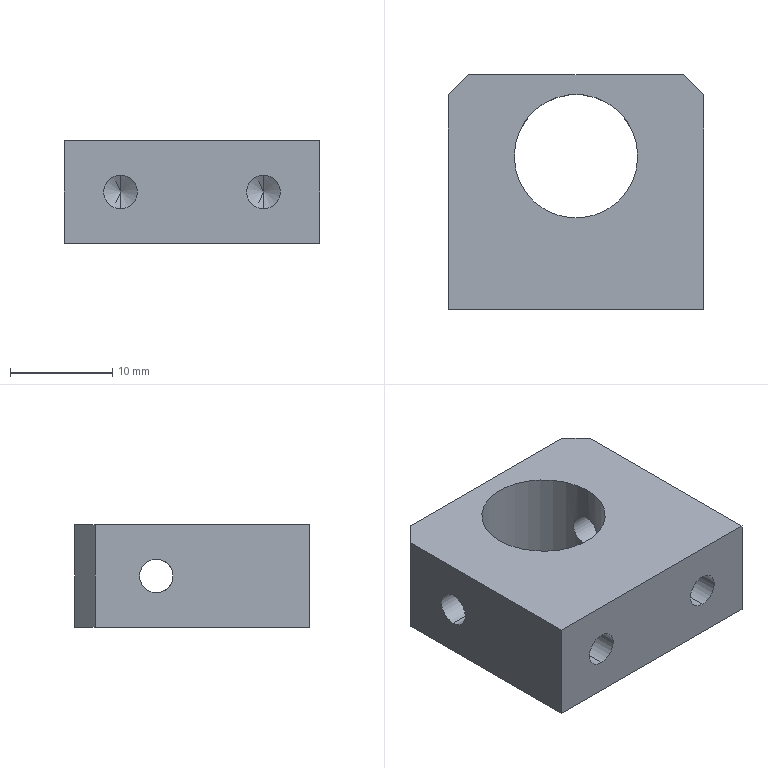Part | SolidWorks | features HoleWzd 2, Chamfer 1, Extrusion 1, ICE 1, MirrorPattern 1 | 1 solid | 22 faces | box 25 x 23 x 10 mm | volume 4270 mm3 | cylinder 10 | plane 8 | cone 4 | commonest cylinder face diameters 3.3 x8 12.1 x2
STEP:
#1=CARTESIAN_POINT('',(6.05,3.5,6.65));
#2=VERTEX_POINT('',#1);
#3=CARTESIAN_POINT('',(6.05,3.5,3.35));
#4=VERTEX_POINT('',#3);
#5=CARTESIAN_POINT('',(6.05,3.5,6.65));
#6=CARTESIAN_POINT('',(6.05,3.284,6.65));
#7=CARTESIAN_POINT('',(6.038,3.066,6.606));
#8=CARTESIAN_POINT('',(6.006,2.768,6.483));
#9=CARTESIAN_POINT('',(5.994,2.671,6.431));
#10=CARTESIAN_POINT('',(5.966,2.492,6.311));
#11=CARTESIAN_POINT('',(5.951,2.41,6.243));
#12=CARTESIAN_POINT('',(5.922,2.258,6.091));
#13=CARTESIAN_POINT('',(5.906,2.188,6.007));
#14=CARTESIAN_POINT('',(5.879,2.069,5.829));
#15=CARTESIAN_POINT('',(5.866,2.018,5.734));
#16=CARTESIAN_POINT('',(5.844,1.935,5.533));
#17=CARTESIAN_POINT('',(5.836,1.903,5.43));
#18=CARTESIAN_POINT('',(5.824,1.861,5.218));
#19=CARTESIAN_POINT('',(5.821,1.85,5.109));
#20=CARTESIAN_POINT('',(5.821,1.85,4.892));
#21=CARTESIAN_POINT('',(5.824,1.861,4.784));
#22=CARTESIAN_POINT('',(5.835,1.903,4.572));
#23=CARTESIAN_POINT('',(5.844,1.935,4.467));
#24=CARTESIAN_POINT('',(5.876,2.059,4.168));
#25=CARTESIAN_POINT('',(5.907,2.181,3.985));
#26=CARTESIAN_POINT('',(5.966,2.484,3.682));
#27=CARTESIAN_POINT('',(5.996,2.667,3.56));
#28=CARTESIAN_POINT('',(6.027,2.965,3.435));
#29=CARTESIAN_POINT('',(6.036,3.07,3.403));
#30=CARTESIAN_POINT('',(6.047,3.283,3.361));
#31=CARTESIAN_POINT('',(6.05,3.39,3.35));
#32=CARTESIAN_POINT('',(6.05,3.5,3.35));
#33=B_SPLINE_CURVE_WITH_KNOTS('',3,(#5,#6,#7,#8,#9,#10,#11,#12,#13,#14,#15,#16,#17,#18,#19,#20,#21,#22,#23,#24,#25,#26,#27,#28,#29,#30,#31,#32),.UNSPECIFIED.,.F.,.F.,(4,2,2,2,2,2,2,2,2,2,2,2,2,4),(0.005183,0.005831,0.006155,0.006479,0.006803,0.007127,0.00745,0.007774,0.008098,0.008422,0.00907,0.009717,0.01004,0.01037),.UNSPECIFIED.);
#34=EDGE_CURVE('',#2,#4,#33,.T.);
#35=ORIENTED_EDGE('',*,*,#34,.F.);
#36=CARTESIAN_POINT('',(12.5,3.5,6.65));
#37=VERTEX_POINT('',#36);
#38=CARTESIAN_POINT('',(12.5,3.5,6.65));
#39=DIRECTION('',(1.,0.,0.));
#40=VECTOR('',#39,1000.);
#41=LINE('',#38,#40);
#42=EDGE_CURVE('',#2,#37,#41,.T.);
#43=ORIENTED_EDGE('',*,*,#42,.T.);
#44=CARTESIAN_POINT('',(12.5,3.5,3.35));
#45=VERTEX_POINT('',#44);
#46=CARTESIAN_POINT('',(12.5,3.5,5.));
#47=DIRECTION('',(1.,0.,0.));
#48=DIRECTION('',(0.,0.,-1.));
#49=AXIS2_PLACEMENT_3D('',#46,#47,#48);
#50=CIRCLE('',#49,1.65);
#51=EDGE_CURVE('',#37,#45,#50,.T.);
#52=ORIENTED_EDGE('',*,*,#51,.T.);
#53=CARTESIAN_POINT('',(12.5,3.5,3.35));
#54=DIRECTION('',(1.,0.,0.));
#55=VECTOR('',#54,1000.);
#56=LINE('',#53,#55);
#57=EDGE_CURVE('',#4,#45,#56,.T.);
#58=ORIENTED_EDGE('',*,*,#57,.F.);
#59=EDGE_LOOP('',(#35,#43,#52,#58));
#60=FACE_OUTER_BOUND('',#59,.T.);
#61=CARTESIAN_POINT('',(12.5,3.5,5.));
#62=DIRECTION('',(1.,0.,0.));
#63=DIRECTION('',(0.,0.,-1.));
#64=AXIS2_PLACEMENT_3D('',#61,#62,#63);
#65=CYLINDRICAL_SURFACE('',#64,1.65);
#66=ADVANCED_FACE('',(#60),#65,.F.);
#67=CARTESIAN_POINT('',(-6.05,3.5,3.35));
#68=VERTEX_POINT('',#67);
#69=CARTESIAN_POINT('',(-6.05,3.5,6.65));
#70=VERTEX_POINT('',#69);
#71=CARTESIAN_POINT('',(-6.05,3.5,3.35));
#72=CARTESIAN_POINT('',(-6.05,3.284,3.35));
#73=CARTESIAN_POINT('',(-6.038,3.066,3.394));
#74=CARTESIAN_POINT('',(-6.006,2.768,3.517));
#75=CARTESIAN_POINT('',(-5.994,2.671,3.569));
#76=CARTESIAN_POINT('',(-5.966,2.492,3.689));
#77=CARTESIAN_POINT('',(-5.951,2.41,3.757));
#78=CARTESIAN_POINT('',(-5.922,2.258,3.909));
#79=CARTESIAN_POINT('',(-5.906,2.188,3.993));
#80=CARTESIAN_POINT('',(-5.879,2.069,4.171));
#81=CARTESIAN_POINT('',(-5.866,2.018,4.266));
#82=CARTESIAN_POINT('',(-5.844,1.935,4.467));
#83=CARTESIAN_POINT('',(-5.836,1.903,4.57));
#84=CARTESIAN_POINT('',(-5.824,1.861,4.782));
#85=CARTESIAN_POINT('',(-5.821,1.85,4.891));
#86=CARTESIAN_POINT('',(-5.821,1.85,5.108));
#87=CARTESIAN_POINT('',(-5.824,1.861,5.216));
#88=CARTESIAN_POINT('',(-5.835,1.903,5.428));
#89=CARTESIAN_POINT('',(-5.844,1.935,5.533));
#90=CARTESIAN_POINT('',(-5.876,2.059,5.832));
#91=CARTESIAN_POINT('',(-5.907,2.181,6.015));
#92=CARTESIAN_POINT('',(-5.966,2.484,6.318));
#93=CARTESIAN_POINT('',(-5.996,2.667,6.44));
#94=CARTESIAN_POINT('',(-6.027,2.965,6.565));
#95=CARTESIAN_POINT('',(-6.036,3.07,6.597));
#96=CARTESIAN_POINT('',(-6.047,3.283,6.639));
#97=CARTESIAN_POINT('',(-6.05,3.39,6.65));
#98=CARTESIAN_POINT('',(-6.05,3.5,6.65));
#99=B_SPLINE_CURVE_WITH_KNOTS('',3,(#71,#72,#73,#74,#75,#76,#77,#78,#79,#80,#81,#82,#83,#84,#85,#86,#87,#88,#89,#90,#91,#92,#93,#94,#95,#96,#97,#98),.UNSPECIFIED.,.F.,.F.,(4,2,2,2,2,2,2,2,2,2,2,2,2,4),(0.005183,0.005831,0.006155,0.006479,0.006803,0.007127,0.00745,0.007774,0.008098,0.008422,0.00907,0.009717,0.01004,0.01037),.UNSPECIFIED.);
#100=EDGE_CURVE('',#68,#70,#99,.T.);
#101=ORIENTED_EDGE('',*,*,#100,.F.);
#102=CARTESIAN_POINT('',(-12.5,3.5,3.35));
#103=VERTEX_POINT('',#102);
#104=CARTESIAN_POINT('',(-12.5,3.5,3.35));
#105=DIRECTION('',(-1.,0.,0.));
#106=VECTOR('',#105,1000.);
#107=LINE('',#104,#106);
#108=EDGE_CURVE('',#68,#103,#107,.T.);
#109=ORIENTED_EDGE('',*,*,#108,.T.);
#110=CARTESIAN_POINT('',(-12.5,3.5,6.65));
#111=VERTEX_POINT('',#110);
#112=CARTESIAN_POINT('',(-12.5,3.5,5.));
#113=DIRECTION('',(-1.,0.,0.));
#114=DIRECTION('',(0.,0.,1.));
#115=AXIS2_PLACEMENT_3D('',#112,#113,#114);
#116=CIRCLE('',#115,1.65);
#117=EDGE_CURVE('',#103,#111,#116,.T.);
#118=ORIENTED_EDGE('',*,*,#117,.T.);
#119=CARTESIAN_POINT('',(-12.5,3.5,6.65));
#120=DIRECTION('',(-1.,0.,0.));
#121=VECTOR('',#120,1000.);
#122=LINE('',#119,#121);
#123=EDGE_CURVE('',#70,#111,#122,.T.);
#124=ORIENTED_EDGE('',*,*,#123,.F.);
#125=EDGE_LOOP('',(#101,#109,#118,#124));
#126=FACE_OUTER_BOUND('',#125,.T.);
#127=CARTESIAN_POINT('',(-12.5,3.5,5.));
#128=DIRECTION('',(-1.,0.,0.));
#129=DIRECTION('',(0.,0.,1.));
#130=AXIS2_PLACEMENT_3D('',#127,#128,#129);
#131=CYLINDRICAL_SURFACE('',#130,1.65);
#132=ADVANCED_FACE('',(#126),#131,.F.);
#133=CARTESIAN_POINT('',(-7.,-1.4,6.65));
#134=VERTEX_POINT('',#133);
#135=CARTESIAN_POINT('',(-7.,-1.4,3.35));
#136=VERTEX_POINT('',#135);
#137=CARTESIAN_POINT('',(-7.,-1.4,5.));
#138=DIRECTION('',(0.,-1.,0.));
#139=DIRECTION('',(0.,0.,-1.));
#140=AXIS2_PLACEMENT_3D('',#137,#138,#139);
#141=CIRCLE('',#140,1.65);
#142=EDGE_CURVE('',#134,#136,#141,.T.);
#143=ORIENTED_EDGE('',*,*,#142,.F.);
#144=CARTESIAN_POINT('',(-7.,-11.5,6.65));
#145=VERTEX_POINT('',#144);
#146=CARTESIAN_POINT('',(-7.,-11.5,6.65));
#147=DIRECTION('',(0.,-1.,0.));
#148=VECTOR('',#147,1000.);
#149=LINE('',#146,#148);
#150=EDGE_CURVE('',#134,#145,#149,.T.);
#151=ORIENTED_EDGE('',*,*,#150,.T.);
#152=CARTESIAN_POINT('',(-7.,-11.5,3.35));
#153=VERTEX_POINT('',#152);
#154=CARTESIAN_POINT('',(-7.,-11.5,5.));
#155=DIRECTION('',(0.,-1.,0.));
#156=DIRECTION('',(0.,0.,-1.));
#157=AXIS2_PLACEMENT_3D('',#154,#155,#156);
#158=CIRCLE('',#157,1.65);
#159=EDGE_CURVE('',#145,#153,#158,.T.);
#160=ORIENTED_EDGE('',*,*,#159,.T.);
#161=CARTESIAN_POINT('',(-7.,-11.5,3.35));
#162=DIRECTION('',(0.,-1.,0.));
#163=VECTOR('',#162,1000.);
#164=LINE('',#161,#163);
#165=EDGE_CURVE('',#136,#153,#164,.T.);
#166=ORIENTED_EDGE('',*,*,#165,.F.);
#167=EDGE_LOOP('',(#143,#151,#160,#166));
#168=FACE_OUTER_BOUND('',#167,.T.);
#169=CARTESIAN_POINT('',(-7.,-11.5,5.));
#170=DIRECTION('',(0.,-1.,0.));
#171=DIRECTION('',(0.,0.,-1.));
#172=AXIS2_PLACEMENT_3D('',#169,#170,#171);
#173=CYLINDRICAL_SURFACE('',#172,1.65);
#174=ADVANCED_FACE('',(#168),#173,.F.);
#175=CARTESIAN_POINT('',(-7.,-0.4086,5.));
#176=VERTEX_POINT('',#175);
#177=CARTESIAN_POINT('',(-7.,-1.4,3.35));
#178=DIRECTION('',(0.,-0.515,-0.8572));
#179=VECTOR('',#178,1000.);
#180=LINE('',#177,#179);
#181=EDGE_CURVE('',#176,#136,#180,.T.);
#182=ORIENTED_EDGE('',*,*,#181,.F.);
#183=CARTESIAN_POINT('',(-7.,-1.4,6.65));
#184=DIRECTION('',(0.,-0.515,0.8572));
#185=VECTOR('',#184,1000.);
#186=LINE('',#183,#185);
#187=EDGE_CURVE('',#176,#134,#186,.T.);
#188=ORIENTED_EDGE('',*,*,#187,.T.);
#189=ORIENTED_EDGE('',*,*,#142,.T.);
#190=EDGE_LOOP('',(#182,#188,#189));
#191=FACE_OUTER_BOUND('',#190,.T.);
#192=CARTESIAN_POINT('',(-7.,-1.4,5.));
#193=DIRECTION('',(0.,-1.,0.));
#194=DIRECTION('',(0.,0.,-1.));
#195=AXIS2_PLACEMENT_3D('',#192,#193,#194);
#196=CONICAL_SURFACE('',#195,1.65,1.03);
#197=ADVANCED_FACE('',(#191),#196,.F.);
#198=CARTESIAN_POINT('',(7.,-1.4,6.65));
#199=VERTEX_POINT('',#198);
#200=CARTESIAN_POINT('',(7.,-1.4,3.35));
#201=VERTEX_POINT('',#200);
#202=CARTESIAN_POINT('',(7.,-1.4,5.));
#203=DIRECTION('',(0.,-1.,0.));
#204=DIRECTION('',(0.,0.,-1.));
#205=AXIS2_PLACEMENT_3D('',#202,#203,#204);
#206=CIRCLE('',#205,1.65);
#207=EDGE_CURVE('',#199,#201,#206,.T.);
#208=ORIENTED_EDGE('',*,*,#207,.F.);
#209=CARTESIAN_POINT('',(7.,-11.5,6.65));
#210=VERTEX_POINT('',#209);
#211=CARTESIAN_POINT('',(7.,-11.5,6.65));
#212=DIRECTION('',(0.,-1.,0.));
#213=VECTOR('',#212,1000.);
#214=LINE('',#211,#213);
#215=EDGE_CURVE('',#199,#210,#214,.T.);
#216=ORIENTED_EDGE('',*,*,#215,.T.);
#217=CARTESIAN_POINT('',(7.,-11.5,3.35));
#218=VERTEX_POINT('',#217);
#219=CARTESIAN_POINT('',(7.,-11.5,5.));
#220=DIRECTION('',(0.,-1.,0.));
#221=DIRECTION('',(0.,0.,-1.));
#222=AXIS2_PLACEMENT_3D('',#219,#220,#221);
#223=CIRCLE('',#222,1.65);
#224=EDGE_CURVE('',#210,#218,#223,.T.);
#225=ORIENTED_EDGE('',*,*,#224,.T.);
#226=CARTESIAN_POINT('',(7.,-11.5,3.35));
#227=DIRECTION('',(0.,-1.,0.));
#228=VECTOR('',#227,1000.);
#229=LINE('',#226,#228);
#230=EDGE_CURVE('',#201,#218,#229,.T.);
#231=ORIENTED_EDGE('',*,*,#230,.F.);
#232=EDGE_LOOP('',(#208,#216,#225,#231));
#233=FACE_OUTER_BOUND('',#232,.T.);
#234=CARTESIAN_POINT('',(7.,-11.5,5.));
#235=DIRECTION('',(0.,-1.,0.));
#236=DIRECTION('',(0.,0.,-1.));
#237=AXIS2_PLACEMENT_3D('',#234,#235,#236);
#238=CYLINDRICAL_SURFACE('',#237,1.65);
#239=ADVANCED_FACE('',(#233),#238,.F.);
#240=CARTESIAN_POINT('',(7.,-0.4086,5.));
#241=VERTEX_POINT('',#240);
#242=CARTESIAN_POINT('',(7.,-1.4,3.35));
#243=DIRECTION('',(0.,-0.515,-0.8572));
#244=VECTOR('',#243,1000.);
#245=LINE('',#242,#244);
#246=EDGE_CURVE('',#241,#201,#245,.T.);
#247=ORIENTED_EDGE('',*,*,#246,.F.);
#248=CARTESIAN_POINT('',(7.,-1.4,6.65));
#249=DIRECTION('',(0.,-0.515,0.8572));
#250=VECTOR('',#249,1000.);
#251=LINE('',#248,#250);
#252=EDGE_CURVE('',#241,#199,#251,.T.);
#253=ORIENTED_EDGE('',*,*,#252,.T.);
#254=ORIENTED_EDGE('',*,*,#207,.T.);
#255=EDGE_LOOP('',(#247,#253,#254));
#256=FACE_OUTER_BOUND('',#255,.T.);
#257=CARTESIAN_POINT('',(7.,-1.4,5.));
#258=DIRECTION('',(0.,-1.,0.));
#259=DIRECTION('',(0.,0.,-1.));
#260=AXIS2_PLACEMENT_3D('',#257,#258,#259);
#261=CONICAL_SURFACE('',#260,1.65,1.03);
#262=ADVANCED_FACE('',(#256),#261,.F.);
#263=CARTESIAN_POINT('',(-6.05,3.5,0.));
#264=VERTEX_POINT('',#263);
#265=CARTESIAN_POINT('',(6.05,3.5,0.));
#266=VERTEX_POINT('',#265);
#267=CARTESIAN_POINT('',(0.,3.5,0.));
#268=DIRECTION('',(0.,0.,1.));
#269=DIRECTION('',(1.,0.,0.));
#270=AXIS2_PLACEMENT_3D('',#267,#268,#269);
#271=CIRCLE('',#270,6.05);
#272=EDGE_CURVE('',#264,#266,#271,.T.);
#273=ORIENTED_EDGE('',*,*,#272,.F.);
#274=CARTESIAN_POINT('',(-6.05,3.5,0.));
#275=DIRECTION('',(0.,0.,1.));
#276=VECTOR('',#275,1000.);
#277=LINE('',#274,#276);
#278=EDGE_CURVE('',#264,#68,#277,.T.);
#279=ORIENTED_EDGE('',*,*,#278,.T.);
#280=ORIENTED_EDGE('',*,*,#100,.T.);
#281=CARTESIAN_POINT('',(-6.05,3.5,10.));
#282=VERTEX_POINT('',#281);
#283=CARTESIAN_POINT('',(-6.05,3.5,0.));
#284=DIRECTION('',(0.,0.,1.));
#285=VECTOR('',#284,1000.);
#286=LINE('',#283,#285);
#287=EDGE_CURVE('',#70,#282,#286,.T.);
#288=ORIENTED_EDGE('',*,*,#287,.T.);
#289=CARTESIAN_POINT('',(6.05,3.5,10.));
#290=VERTEX_POINT('',#289);
#291=CARTESIAN_POINT('',(0.,3.5,10.));
#292=DIRECTION('',(0.,0.,1.));
#293=DIRECTION('',(1.,0.,0.));
#294=AXIS2_PLACEMENT_3D('',#291,#292,#293);
#295=CIRCLE('',#294,6.05);
#296=EDGE_CURVE('',#282,#290,#295,.T.);
#297=ORIENTED_EDGE('',*,*,#296,.T.);
#298=CARTESIAN_POINT('',(6.05,3.5,0.));
#299=DIRECTION('',(0.,0.,1.));
#300=VECTOR('',#299,1000.);
#301=LINE('',#298,#300);
#302=EDGE_CURVE('',#2,#290,#301,.T.);
#303=ORIENTED_EDGE('',*,*,#302,.F.);
#304=ORIENTED_EDGE('',*,*,#34,.T.);
#305=CARTESIAN_POINT('',(6.05,3.5,0.));
#306=DIRECTION('',(0.,0.,1.));
#307=VECTOR('',#306,1000.);
#308=LINE('',#305,#307);
#309=EDGE_CURVE('',#266,#4,#308,.T.);
#310=ORIENTED_EDGE('',*,*,#309,.F.);
#311=EDGE_LOOP('',(#273,#279,#280,#288,#297,#303,#304,#310));
#312=FACE_OUTER_BOUND('',#311,.T.);
#313=CARTESIAN_POINT('',(0.,3.5,0.));
#314=DIRECTION('',(0.,0.,1.));
#315=DIRECTION('',(1.,0.,0.));
#316=AXIS2_PLACEMENT_3D('',#313,#314,#315);
#317=CYLINDRICAL_SURFACE('',#316,6.05);
#318=ADVANCED_FACE('',(#312),#317,.F.);
#319=CARTESIAN_POINT('',(12.5,3.5,5.));
#320=DIRECTION('',(1.,0.,0.));
#321=DIRECTION('',(0.,0.,-1.));
#322=AXIS2_PLACEMENT_3D('',#319,#320,#321);
#323=CIRCLE('',#322,1.65);
#324=EDGE_CURVE('',#45,#37,#323,.T.);
#325=ORIENTED_EDGE('',*,*,#324,.F.);
#326=ORIENTED_EDGE('',*,*,#51,.F.);
#327=EDGE_LOOP('',(#325,#326));
#328=FACE_BOUND('',#327,.T.);
#329=CARTESIAN_POINT('',(12.5,-11.5,0.));
#330=VERTEX_POINT('',#329);
#331=CARTESIAN_POINT('',(12.5,9.5,0.));
#332=VERTEX_POINT('',#331);
#333=CARTESIAN_POINT('',(12.5,-11.5,0.));
#334=DIRECTION('',(0.,1.,0.));
#335=VECTOR('',#334,1000.);
#336=LINE('',#333,#335);
#337=EDGE_CURVE('',#330,#332,#336,.T.);
#338=ORIENTED_EDGE('',*,*,#337,.T.);
#339=CARTESIAN_POINT('',(12.5,9.5,10.));
#340=VERTEX_POINT('',#339);
#341=CARTESIAN_POINT('',(12.5,9.5,10.));
#342=DIRECTION('',(0.,0.,1.));
#343=VECTOR('',#342,1000.);
#344=LINE('',#341,#343);
#345=EDGE_CURVE('',#332,#340,#344,.T.);
#346=ORIENTED_EDGE('',*,*,#345,.T.);
#347=CARTESIAN_POINT('',(12.5,-11.5,10.));
#348=VERTEX_POINT('',#347);
#349=CARTESIAN_POINT('',(12.5,-11.5,10.));
#350=DIRECTION('',(0.,1.,0.));
#351=VECTOR('',#350,1000.);
#352=LINE('',#349,#351);
#353=EDGE_CURVE('',#348,#340,#352,.T.);
#354=ORIENTED_EDGE('',*,*,#353,.F.);
#355=CARTESIAN_POINT('',(12.5,-11.5,10.));
#356=DIRECTION('',(0.,0.,-1.));
#357=VECTOR('',#356,1000.);
#358=LINE('',#355,#357);
#359=EDGE_CURVE('',#348,#330,#358,.T.);
#360=ORIENTED_EDGE('',*,*,#359,.T.);
#361=EDGE_LOOP('',(#338,#346,#354,#360));
#362=FACE_OUTER_BOUND('',#361,.T.);
#363=CARTESIAN_POINT('',(12.5,-11.5,10.));
#364=DIRECTION('',(-1.,0.,0.));
#365=DIRECTION('',(0.,0.,1.));
#366=AXIS2_PLACEMENT_3D('',#363,#364,#365);
#367=PLANE('',#366);
#368=ADVANCED_FACE('',(#328,#362),#367,.F.);
#369=CARTESIAN_POINT('',(10.5,11.5,10.));
#370=VERTEX_POINT('',#369);
#371=CARTESIAN_POINT('',(-10.5,11.5,10.));
#372=VERTEX_POINT('',#371);
#373=CARTESIAN_POINT('',(-12.5,11.5,10.));
#374=DIRECTION('',(-1.,0.,0.));
#375=VECTOR('',#374,1000.);
#376=LINE('',#373,#375);
#377=EDGE_CURVE('',#370,#372,#376,.T.);
#378=ORIENTED_EDGE('',*,*,#377,.F.);
#379=CARTESIAN_POINT('',(10.5,11.5,0.));
#380=VERTEX_POINT('',#379);
#381=CARTESIAN_POINT('',(10.5,11.5,10.));
#382=DIRECTION('',(0.,0.,-1.));
#383=VECTOR('',#382,1000.);
#384=LINE('',#381,#383);
#385=EDGE_CURVE('',#370,#380,#384,.T.);
#386=ORIENTED_EDGE('',*,*,#385,.T.);
#387=CARTESIAN_POINT('',(-10.5,11.5,0.));
#388=VERTEX_POINT('',#387);
#389=CARTESIAN_POINT('',(-12.5,11.5,0.));
#390=DIRECTION('',(-1.,0.,0.));
#391=VECTOR('',#390,1000.);
#392=LINE('',#389,#391);
#393=EDGE_CURVE('',#380,#388,#392,.T.);
#394=ORIENTED_EDGE('',*,*,#393,.T.);
#395=CARTESIAN_POINT('',(-10.5,11.5,10.));
#396=DIRECTION('',(0.,0.,1.));
#397=VECTOR('',#396,1000.);
#398=LINE('',#395,#397);
#399=EDGE_CURVE('',#388,#372,#398,.T.);
#400=ORIENTED_EDGE('',*,*,#399,.T.);
#401=EDGE_LOOP('',(#378,#386,#394,#400));
#402=FACE_OUTER_BOUND('',#401,.T.);
#403=CARTESIAN_POINT('',(-12.5,11.5,10.));
#404=DIRECTION('',(0.,-1.,0.));
#405=DIRECTION('',(0.,0.,-1.));
#406=AXIS2_PLACEMENT_3D('',#403,#404,#405);
#407=PLANE('',#406);
#408=ADVANCED_FACE('',(#402),#407,.F.);
#409=CARTESIAN_POINT('',(-12.5,3.5,5.));
#410=DIRECTION('',(-1.,0.,0.));
#411=DIRECTION('',(0.,0.,1.));
#412=AXIS2_PLACEMENT_3D('',#409,#410,#411);
#413=CIRCLE('',#412,1.65);
#414=EDGE_CURVE('',#111,#103,#413,.T.);
#415=ORIENTED_EDGE('',*,*,#414,.F.);
#416=ORIENTED_EDGE('',*,*,#117,.F.);
#417=EDGE_LOOP('',(#415,#416));
#418=FACE_BOUND('',#417,.T.);
#419=CARTESIAN_POINT('',(-12.5,9.5,10.));
#420=VERTEX_POINT('',#419);
#421=CARTESIAN_POINT('',(-12.5,-11.5,10.));
#422=VERTEX_POINT('',#421);
#423=CARTESIAN_POINT('',(-12.5,-11.5,10.));
#424=DIRECTION('',(0.,-1.,0.));
#425=VECTOR('',#424,1000.);
#426=LINE('',#423,#425);
#427=EDGE_CURVE('',#420,#422,#426,.T.);
#428=ORIENTED_EDGE('',*,*,#427,.F.);
#429=CARTESIAN_POINT('',(-12.5,9.5,0.));
#430=VERTEX_POINT('',#429);
#431=CARTESIAN_POINT('',(-12.5,9.5,10.));
#432=DIRECTION('',(0.,0.,-1.));
#433=VECTOR('',#432,1000.);
#434=LINE('',#431,#433);
#435=EDGE_CURVE('',#420,#430,#434,.T.);
#436=ORIENTED_EDGE('',*,*,#435,.T.);
#437=CARTESIAN_POINT('',(-12.5,-11.5,0.));
#438=VERTEX_POINT('',#437);
#439=CARTESIAN_POINT('',(-12.5,-11.5,0.));
#440=DIRECTION('',(0.,-1.,0.));
#441=VECTOR('',#440,1000.);
#442=LINE('',#439,#441);
#443=EDGE_CURVE('',#430,#438,#442,.T.);
#444=ORIENTED_EDGE('',*,*,#443,.T.);
#445=CARTESIAN_POINT('',(-12.5,-11.5,10.));
#446=DIRECTION('',(0.,0.,-1.));
#447=VECTOR('',#446,1000.);
#448=LINE('',#445,#447);
#449=EDGE_CURVE('',#422,#438,#448,.T.);
#450=ORIENTED_EDGE('',*,*,#449,.F.);
#451=EDGE_LOOP('',(#428,#436,#444,#450));
#452=FACE_OUTER_BOUND('',#451,.T.);
#453=CARTESIAN_POINT('',(-12.5,-11.5,10.));
#454=DIRECTION('',(1.,0.,0.));
#455=DIRECTION('',(0.,0.,-1.));
#456=AXIS2_PLACEMENT_3D('',#453,#454,#455);
#457=PLANE('',#456);
#458=ADVANCED_FACE('',(#418,#452),#457,.F.);
#459=CARTESIAN_POINT('',(-7.,-11.5,5.));
#460=DIRECTION('',(0.,-1.,0.));
#461=DIRECTION('',(0.,0.,-1.));
#462=AXIS2_PLACEMENT_3D('',#459,#460,#461);
#463=CIRCLE('',#462,1.65);
#464=EDGE_CURVE('',#153,#145,#463,.T.);
#465=ORIENTED_EDGE('',*,*,#464,.F.);
#466=ORIENTED_EDGE('',*,*,#159,.F.);
#467=EDGE_LOOP('',(#465,#466));
#468=FACE_BOUND('',#467,.T.);
#469=CARTESIAN_POINT('',(7.,-11.5,5.));
#470=DIRECTION('',(0.,-1.,0.));
#471=DIRECTION('',(0.,0.,-1.));
#472=AXIS2_PLACEMENT_3D('',#469,#470,#471);
#473=CIRCLE('',#472,1.65);
#474=EDGE_CURVE('',#218,#210,#473,.T.);
#475=ORIENTED_EDGE('',*,*,#474,.F.);
#476=ORIENTED_EDGE('',*,*,#224,.F.);
#477=EDGE_LOOP('',(#475,#476));
#478=FACE_BOUND('',#477,.T.);
#479=CARTESIAN_POINT('',(-12.5,-11.5,0.));
#480=DIRECTION('',(1.,0.,0.));
#481=VECTOR('',#480,1000.);
#482=LINE('',#479,#481);
#483=EDGE_CURVE('',#438,#330,#482,.T.);
#484=ORIENTED_EDGE('',*,*,#483,.T.);
#485=ORIENTED_EDGE('',*,*,#359,.F.);
#486=CARTESIAN_POINT('',(-12.5,-11.5,10.));
#487=DIRECTION('',(1.,0.,0.));
#488=VECTOR('',#487,1000.);
#489=LINE('',#486,#488);
#490=EDGE_CURVE('',#422,#348,#489,.T.);
#491=ORIENTED_EDGE('',*,*,#490,.F.);
#492=ORIENTED_EDGE('',*,*,#449,.T.);
#493=EDGE_LOOP('',(#484,#485,#491,#492));
#494=FACE_OUTER_BOUND('',#493,.T.);
#495=CARTESIAN_POINT('',(-12.5,-11.5,10.));
#496=DIRECTION('',(0.,1.,0.));
#497=DIRECTION('',(0.,0.,1.));
#498=AXIS2_PLACEMENT_3D('',#495,#496,#497);
#499=PLANE('',#498);
#500=ADVANCED_FACE('',(#468,#478,#494),#499,.F.);
#501=CARTESIAN_POINT('',(0.,3.5,10.));
#502=DIRECTION('',(0.,0.,1.));
#503=DIRECTION('',(1.,0.,0.));
#504=AXIS2_PLACEMENT_3D('',#501,#502,#503);
#505=CIRCLE('',#504,6.05);
#506=EDGE_CURVE('',#290,#282,#505,.T.);
#507=ORIENTED_EDGE('',*,*,#506,.F.);
#508=ORIENTED_EDGE('',*,*,#296,.F.);
#509=EDGE_LOOP('',(#507,#508));
#510=FACE_BOUND('',#509,.T.);
#511=ORIENTED_EDGE('',*,*,#353,.T.);
#512=CARTESIAN_POINT('',(10.5,11.5,10.));
#513=DIRECTION('',(-0.7071,0.7071,0.));
#514=VECTOR('',#513,1000.);
#515=LINE('',#512,#514);
#516=EDGE_CURVE('',#340,#370,#515,.T.);
#517=ORIENTED_EDGE('',*,*,#516,.T.);
#518=ORIENTED_EDGE('',*,*,#377,.T.);
#519=CARTESIAN_POINT('',(-12.5,9.5,10.));
#520=DIRECTION('',(-0.7071,-0.7071,0.));
#521=VECTOR('',#520,1000.);
#522=LINE('',#519,#521);
#523=EDGE_CURVE('',#372,#420,#522,.T.);
#524=ORIENTED_EDGE('',*,*,#523,.T.);
#525=ORIENTED_EDGE('',*,*,#427,.T.);
#526=ORIENTED_EDGE('',*,*,#490,.T.);
#527=EDGE_LOOP('',(#511,#517,#518,#524,#525,#526));
#528=FACE_OUTER_BOUND('',#527,.T.);
#529=CARTESIAN_POINT('',(12.5,11.5,10.));
#530=DIRECTION('',(0.,0.,-1.));
#531=DIRECTION('',(-1.,0.,0.));
#532=AXIS2_PLACEMENT_3D('',#529,#530,#531);
#533=PLANE('',#532);
#534=ADVANCED_FACE('',(#510,#528),#533,.F.);
#535=CARTESIAN_POINT('',(0.,3.5,0.));
#536=DIRECTION('',(0.,0.,1.));
#537=DIRECTION('',(1.,0.,0.));
#538=AXIS2_PLACEMENT_3D('',#535,#536,#537);
#539=CIRCLE('',#538,6.05);
#540=EDGE_CURVE('',#266,#264,#539,.T.);
#541=ORIENTED_EDGE('',*,*,#540,.T.);
#542=ORIENTED_EDGE('',*,*,#272,.T.);
#543=EDGE_LOOP('',(#541,#542));
#544=FACE_BOUND('',#543,.T.);
#545=ORIENTED_EDGE('',*,*,#393,.F.);
#546=CARTESIAN_POINT('',(11.5,10.5,0.));
#547=DIRECTION('',(0.7071,-0.7071,0.));
#548=VECTOR('',#547,1000.);
#549=LINE('',#546,#548);
#550=EDGE_CURVE('',#380,#332,#549,.T.);
#551=ORIENTED_EDGE('',*,*,#550,.T.);
#552=ORIENTED_EDGE('',*,*,#337,.F.);
#553=ORIENTED_EDGE('',*,*,#483,.F.);
#554=ORIENTED_EDGE('',*,*,#443,.F.);
#555=CARTESIAN_POINT('',(1.,23.,0.));
#556=DIRECTION('',(0.7071,0.7071,0.));
#557=VECTOR('',#556,1000.);
#558=LINE('',#555,#557);
#559=EDGE_CURVE('',#430,#388,#558,.T.);
#560=ORIENTED_EDGE('',*,*,#559,.T.);
#561=EDGE_LOOP('',(#545,#551,#552,#553,#554,#560));
#562=FACE_OUTER_BOUND('',#561,.T.);
#563=CARTESIAN_POINT('',(12.5,11.5,0.));
#564=DIRECTION('',(0.,0.,-1.));
#565=DIRECTION('',(-1.,0.,0.));
#566=AXIS2_PLACEMENT_3D('',#563,#564,#565);
#567=PLANE('',#566);
#568=ADVANCED_FACE('',(#544,#562),#567,.T.);
#569=ORIENTED_EDGE('',*,*,#278,.F.);
#570=ORIENTED_EDGE('',*,*,#540,.F.);
#571=ORIENTED_EDGE('',*,*,#309,.T.);
#572=CARTESIAN_POINT('',(6.05,3.5,3.35));
#573=CARTESIAN_POINT('',(6.05,3.61,3.35));
#574=CARTESIAN_POINT('',(6.047,3.717,3.361));
#575=CARTESIAN_POINT('',(6.036,3.929,3.403));
#576=CARTESIAN_POINT('',(6.027,4.034,3.435));
#577=CARTESIAN_POINT('',(6.006,4.234,3.518));
#578=CARTESIAN_POINT('',(5.994,4.328,3.569));
#579=CARTESIAN_POINT('',(5.966,4.507,3.689));
#580=CARTESIAN_POINT('',(5.951,4.591,3.758));
#581=CARTESIAN_POINT('',(5.907,4.818,3.985));
#582=CARTESIAN_POINT('',(5.876,4.941,4.168));
#583=CARTESIAN_POINT('',(5.834,5.106,4.565));
#584=CARTESIAN_POINT('',(5.821,5.15,4.783));
#585=CARTESIAN_POINT('',(5.821,5.15,5.107));
#586=CARTESIAN_POINT('',(5.824,5.139,5.217));
#587=CARTESIAN_POINT('',(5.836,5.097,5.429));
#588=CARTESIAN_POINT('',(5.844,5.065,5.533));
#589=CARTESIAN_POINT('',(5.877,4.941,5.833));
#590=CARTESIAN_POINT('',(5.907,4.819,6.014));
#591=CARTESIAN_POINT('',(5.951,4.59,6.243));
#592=CARTESIAN_POINT('',(5.966,4.507,6.311));
#593=CARTESIAN_POINT('',(5.994,4.329,6.431));
#594=CARTESIAN_POINT('',(6.006,4.232,6.483));
#595=CARTESIAN_POINT('',(6.027,4.033,6.565));
#596=CARTESIAN_POINT('',(6.036,3.93,6.597));
#597=CARTESIAN_POINT('',(6.047,3.718,6.639));
#598=CARTESIAN_POINT('',(6.05,3.608,6.65));
#599=CARTESIAN_POINT('',(6.05,3.5,6.65));
#600=B_SPLINE_CURVE_WITH_KNOTS('',3,(#572,#573,#574,#575,#576,#577,#578,#579,#580,#581,#582,#583,#584,#585,#586,#587,#588,#589,#590,#591,#592,#593,#594,#595,#596,#597,#598,#599),.UNSPECIFIED.,.F.,.F.,(4,2,2,2,2,2,2,2,2,2,2,2,2,4),(0.,0.000324,0.0006479,0.0009719,0.001296,0.001944,0.002592,0.002916,0.00324,0.003887,0.004211,0.004535,0.004859,0.005183),.UNSPECIFIED.);
#601=EDGE_CURVE('',#4,#2,#600,.T.);
#602=ORIENTED_EDGE('',*,*,#601,.T.);
#603=ORIENTED_EDGE('',*,*,#302,.T.);
#604=ORIENTED_EDGE('',*,*,#506,.T.);
#605=ORIENTED_EDGE('',*,*,#287,.F.);
#606=CARTESIAN_POINT('',(-6.05,3.5,6.65));
#607=CARTESIAN_POINT('',(-6.05,3.61,6.65));
#608=CARTESIAN_POINT('',(-6.047,3.717,6.639));
#609=CARTESIAN_POINT('',(-6.036,3.929,6.597));
#610=CARTESIAN_POINT('',(-6.027,4.034,6.565));
#611=CARTESIAN_POINT('',(-6.006,4.234,6.482));
#612=CARTESIAN_POINT('',(-5.994,4.328,6.431));
#613=CARTESIAN_POINT('',(-5.966,4.507,6.311));
#614=CARTESIAN_POINT('',(-5.951,4.591,6.242));
#615=CARTESIAN_POINT('',(-5.907,4.818,6.015));
#616=CARTESIAN_POINT('',(-5.876,4.941,5.832));
#617=CARTESIAN_POINT('',(-5.834,5.106,5.435));
#618=CARTESIAN_POINT('',(-5.821,5.15,5.217));
#619=CARTESIAN_POINT('',(-5.821,5.15,4.893));
#620=CARTESIAN_POINT('',(-5.824,5.139,4.783));
#621=CARTESIAN_POINT('',(-5.836,5.097,4.571));
#622=CARTESIAN_POINT('',(-5.844,5.065,4.467));
#623=CARTESIAN_POINT('',(-5.877,4.941,4.167));
#624=CARTESIAN_POINT('',(-5.907,4.819,3.986));
#625=CARTESIAN_POINT('',(-5.951,4.59,3.757));
#626=CARTESIAN_POINT('',(-5.966,4.507,3.689));
#627=CARTESIAN_POINT('',(-5.994,4.329,3.569));
#628=CARTESIAN_POINT('',(-6.006,4.232,3.517));
#629=CARTESIAN_POINT('',(-6.027,4.033,3.435));
#630=CARTESIAN_POINT('',(-6.036,3.93,3.403));
#631=CARTESIAN_POINT('',(-6.047,3.718,3.361));
#632=CARTESIAN_POINT('',(-6.05,3.608,3.35));
#633=CARTESIAN_POINT('',(-6.05,3.5,3.35));
#634=B_SPLINE_CURVE_WITH_KNOTS('',3,(#606,#607,#608,#609,#610,#611,#612,#613,#614,#615,#616,#617,#618,#619,#620,#621,#622,#623,#624,#625,#626,#627,#628,#629,#630,#631,#632,#633),.UNSPECIFIED.,.F.,.F.,(4,2,2,2,2,2,2,2,2,2,2,2,2,4),(0.,0.000324,0.0006479,0.0009719,0.001296,0.001944,0.002592,0.002916,0.00324,0.003887,0.004211,0.004535,0.004859,0.005183),.UNSPECIFIED.);
#635=EDGE_CURVE('',#70,#68,#634,.T.);
#636=ORIENTED_EDGE('',*,*,#635,.T.);
#637=EDGE_LOOP('',(#569,#570,#571,#602,#603,#604,#605,#636));
#638=FACE_OUTER_BOUND('',#637,.T.);
#639=CARTESIAN_POINT('',(0.,3.5,0.));
#640=DIRECTION('',(0.,0.,1.));
#641=DIRECTION('',(1.,0.,0.));
#642=AXIS2_PLACEMENT_3D('',#639,#640,#641);
#643=CYLINDRICAL_SURFACE('',#642,6.05);
#644=ADVANCED_FACE('',(#638),#643,.F.);
#645=ORIENTED_EDGE('',*,*,#516,.F.);
#646=ORIENTED_EDGE('',*,*,#345,.F.);
#647=ORIENTED_EDGE('',*,*,#550,.F.);
#648=ORIENTED_EDGE('',*,*,#385,.F.);
#649=EDGE_LOOP('',(#645,#646,#647,#648));
#650=FACE_OUTER_BOUND('',#649,.T.);
#651=CARTESIAN_POINT('',(10.5,11.5,10.));
#652=DIRECTION('',(-0.7071,-0.7071,0.));
#653=DIRECTION('',(0.7071,-0.7071,0.));
#654=AXIS2_PLACEMENT_3D('',#651,#652,#653);
#655=PLANE('',#654);
#656=ADVANCED_FACE('',(#650),#655,.F.);
#657=ORIENTED_EDGE('',*,*,#523,.F.);
#658=ORIENTED_EDGE('',*,*,#399,.F.);
#659=ORIENTED_EDGE('',*,*,#559,.F.);
#660=ORIENTED_EDGE('',*,*,#435,.F.);
#661=EDGE_LOOP('',(#657,#658,#659,#660));
#662=FACE_OUTER_BOUND('',#661,.T.);
#663=CARTESIAN_POINT('',(-12.5,9.5,10.));
#664=DIRECTION('',(0.7071,-0.7071,0.));
#665=DIRECTION('',(0.7071,0.7071,0.));
#666=AXIS2_PLACEMENT_3D('',#663,#664,#665);
#667=PLANE('',#666);
#668=ADVANCED_FACE('',(#662),#667,.F.);
#669=ORIENTED_EDGE('',*,*,#252,.F.);
#670=ORIENTED_EDGE('',*,*,#246,.T.);
#671=CARTESIAN_POINT('',(7.,-1.4,5.));
#672=DIRECTION('',(0.,-1.,0.));
#673=DIRECTION('',(0.,0.,-1.));
#674=AXIS2_PLACEMENT_3D('',#671,#672,#673);
#675=CIRCLE('',#674,1.65);
#676=EDGE_CURVE('',#201,#199,#675,.T.);
#677=ORIENTED_EDGE('',*,*,#676,.T.);
#678=EDGE_LOOP('',(#669,#670,#677));
#679=FACE_OUTER_BOUND('',#678,.T.);
#680=CARTESIAN_POINT('',(7.,-1.4,5.));
#681=DIRECTION('',(0.,-1.,0.));
#682=DIRECTION('',(0.,0.,-1.));
#683=AXIS2_PLACEMENT_3D('',#680,#681,#682);
#684=CONICAL_SURFACE('',#683,1.65,1.03);
#685=ADVANCED_FACE('',(#679),#684,.F.);
#686=ORIENTED_EDGE('',*,*,#215,.F.);
#687=ORIENTED_EDGE('',*,*,#676,.F.);
#688=ORIENTED_EDGE('',*,*,#230,.T.);
#689=ORIENTED_EDGE('',*,*,#474,.T.);
#690=EDGE_LOOP('',(#686,#687,#688,#689));
#691=FACE_OUTER_BOUND('',#690,.T.);
#692=CARTESIAN_POINT('',(7.,-11.5,5.));
#693=DIRECTION('',(0.,-1.,0.));
#694=DIRECTION('',(0.,0.,-1.));
#695=AXIS2_PLACEMENT_3D('',#692,#693,#694);
#696=CYLINDRICAL_SURFACE('',#695,1.65);
#697=ADVANCED_FACE('',(#691),#696,.F.);
#698=ORIENTED_EDGE('',*,*,#187,.F.);
#699=ORIENTED_EDGE('',*,*,#181,.T.);
#700=CARTESIAN_POINT('',(-7.,-1.4,5.));
#701=DIRECTION('',(0.,-1.,0.));
#702=DIRECTION('',(0.,0.,-1.));
#703=AXIS2_PLACEMENT_3D('',#700,#701,#702);
#704=CIRCLE('',#703,1.65);
#705=EDGE_CURVE('',#136,#134,#704,.T.);
#706=ORIENTED_EDGE('',*,*,#705,.T.);
#707=EDGE_LOOP('',(#698,#699,#706));
#708=FACE_OUTER_BOUND('',#707,.T.);
#709=CARTESIAN_POINT('',(-7.,-1.4,5.));
#710=DIRECTION('',(0.,-1.,0.));
#711=DIRECTION('',(0.,0.,-1.));
#712=AXIS2_PLACEMENT_3D('',#709,#710,#711);
#713=CONICAL_SURFACE('',#712,1.65,1.03);
#714=ADVANCED_FACE('',(#708),#713,.F.);
#715=ORIENTED_EDGE('',*,*,#150,.F.);
#716=ORIENTED_EDGE('',*,*,#705,.F.);
#717=ORIENTED_EDGE('',*,*,#165,.T.);
#718=ORIENTED_EDGE('',*,*,#464,.T.);
#719=EDGE_LOOP('',(#715,#716,#717,#718));
#720=FACE_OUTER_BOUND('',#719,.T.);
#721=CARTESIAN_POINT('',(-7.,-11.5,5.));
#722=DIRECTION('',(0.,-1.,0.));
#723=DIRECTION('',(0.,0.,-1.));
#724=AXIS2_PLACEMENT_3D('',#721,#722,#723);
#725=CYLINDRICAL_SURFACE('',#724,1.65);
#726=ADVANCED_FACE('',(#720),#725,.F.);
#727=ORIENTED_EDGE('',*,*,#108,.F.);
#728=ORIENTED_EDGE('',*,*,#635,.F.);
#729=ORIENTED_EDGE('',*,*,#123,.T.);
#730=ORIENTED_EDGE('',*,*,#414,.T.);
#731=EDGE_LOOP('',(#727,#728,#729,#730));
#732=FACE_OUTER_BOUND('',#731,.T.);
#733=CARTESIAN_POINT('',(-12.5,3.5,5.));
#734=DIRECTION('',(-1.,0.,0.));
#735=DIRECTION('',(0.,0.,1.));
#736=AXIS2_PLACEMENT_3D('',#733,#734,#735);
#737=CYLINDRICAL_SURFACE('',#736,1.65);
#738=ADVANCED_FACE('',(#732),#737,.F.);
#739=ORIENTED_EDGE('',*,*,#42,.F.);
#740=ORIENTED_EDGE('',*,*,#601,.F.);
#741=ORIENTED_EDGE('',*,*,#57,.T.);
#742=ORIENTED_EDGE('',*,*,#324,.T.);
#743=EDGE_LOOP('',(#739,#740,#741,#742));
#744=FACE_OUTER_BOUND('',#743,.T.);
#745=CARTESIAN_POINT('',(12.5,3.5,5.));
#746=DIRECTION('',(1.,0.,0.));
#747=DIRECTION('',(0.,0.,-1.));
#748=AXIS2_PLACEMENT_3D('',#745,#746,#747);
#749=CYLINDRICAL_SURFACE('',#748,1.65);
#750=ADVANCED_FACE('',(#744),#749,.F.);
#751=CLOSED_SHELL('',(#66,#132,#174,#197,#239,#262,#318,#368,#408,#458,#500,#534,#568,#644,#656,#668,#685,#697,#714,#726,#738,#750));
#752=MANIFOLD_SOLID_BREP('',#751);
#753=CARTESIAN_POINT('',(0.,0.,0.));
#754=DIRECTION('',(0.,0.,1.));
#755=DIRECTION('',(1.,0.,0.));
#756=AXIS2_PLACEMENT_3D('',#753,#754,#755);
#757=(LENGTH_UNIT()NAMED_UNIT(*)SI_UNIT(.MILLI.,.METRE.));
#758=UNCERTAINTY_MEASURE_WITH_UNIT(LENGTH_MEASURE(0.00001),#757,'','');
#759=(NAMED_UNIT(*)PLANE_ANGLE_UNIT()SI_UNIT($,.RADIAN.));
#760=(NAMED_UNIT(*)SI_UNIT($,.STERADIAN.)SOLID_ANGLE_UNIT());
#761=(GEOMETRIC_REPRESENTATION_CONTEXT(3)GLOBAL_UNCERTAINTY_ASSIGNED_CONTEXT((#758))GLOBAL_UNIT_ASSIGNED_CONTEXT((#757,#759,#760))REPRESENTATION_CONTEXT('',''));
#762=ADVANCED_BREP_SHAPE_REPRESENTATION('',(#752,#756),#761);